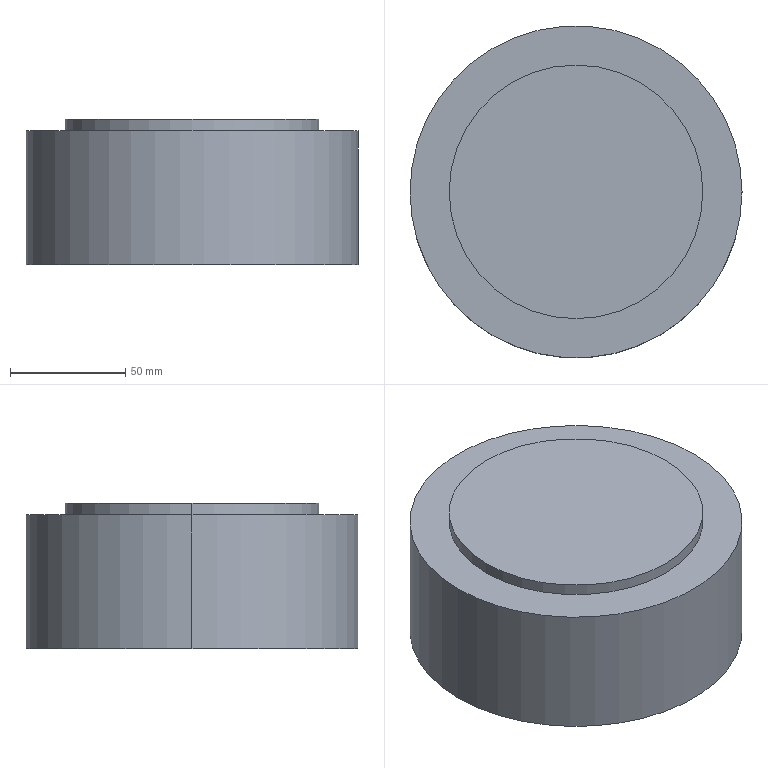Part | SolidWorks | features Extrusion 1, ICE 1 | 1 solid | 7 faces | box 144 x 144 x 63 mm | volume 992106 mm3 | cylinder 4 | plane 3 | commonest cylinder face diameters 110 x2 144 x2
STEP:
#1=CARTESIAN_POINT('',(55.,0.,63.));
#2=VERTEX_POINT('',#1);
#3=CARTESIAN_POINT('',(-55.,0.,63.));
#4=VERTEX_POINT('',#3);
#5=CARTESIAN_POINT('',(0.,0.,63.));
#6=DIRECTION('',(0.,0.,1.));
#7=DIRECTION('',(1.,0.,0.));
#8=AXIS2_PLACEMENT_3D('',#5,#6,#7);
#9=CIRCLE('',#8,55.);
#10=EDGE_CURVE('',#2,#4,#9,.T.);
#11=ORIENTED_EDGE('',*,*,#10,.F.);
#12=CARTESIAN_POINT('',(55.,0.,58.));
#13=VERTEX_POINT('',#12);
#14=CARTESIAN_POINT('',(55.,0.,63.));
#15=DIRECTION('',(0.,0.,-1.));
#16=VECTOR('',#15,1000.);
#17=LINE('',#14,#16);
#18=EDGE_CURVE('',#2,#13,#17,.T.);
#19=ORIENTED_EDGE('',*,*,#18,.T.);
#20=CARTESIAN_POINT('',(-55.,0.,58.));
#21=VERTEX_POINT('',#20);
#22=CARTESIAN_POINT('',(0.,0.,58.));
#23=DIRECTION('',(0.,0.,1.));
#24=DIRECTION('',(1.,0.,0.));
#25=AXIS2_PLACEMENT_3D('',#22,#23,#24);
#26=CIRCLE('',#25,55.);
#27=EDGE_CURVE('',#13,#21,#26,.T.);
#28=ORIENTED_EDGE('',*,*,#27,.T.);
#29=CARTESIAN_POINT('',(-55.,0.,63.));
#30=DIRECTION('',(0.,0.,-1.));
#31=VECTOR('',#30,1000.);
#32=LINE('',#29,#31);
#33=EDGE_CURVE('',#4,#21,#32,.T.);
#34=ORIENTED_EDGE('',*,*,#33,.F.);
#35=EDGE_LOOP('',(#11,#19,#28,#34));
#36=FACE_OUTER_BOUND('',#35,.T.);
#37=CARTESIAN_POINT('',(0.,0.,63.));
#38=DIRECTION('',(0.,0.,-1.));
#39=DIRECTION('',(-1.,0.,0.));
#40=AXIS2_PLACEMENT_3D('',#37,#38,#39);
#41=CYLINDRICAL_SURFACE('',#40,55.);
#42=ADVANCED_FACE('',(#36),#41,.T.);
#43=CARTESIAN_POINT('',(72.,0.,58.));
#44=VERTEX_POINT('',#43);
#45=CARTESIAN_POINT('',(-72.,0.,58.));
#46=VERTEX_POINT('',#45);
#47=CARTESIAN_POINT('',(0.,0.,58.));
#48=DIRECTION('',(0.,0.,1.));
#49=DIRECTION('',(1.,0.,0.));
#50=AXIS2_PLACEMENT_3D('',#47,#48,#49);
#51=CIRCLE('',#50,72.);
#52=EDGE_CURVE('',#44,#46,#51,.T.);
#53=ORIENTED_EDGE('',*,*,#52,.F.);
#54=CARTESIAN_POINT('',(72.,0.,0.));
#55=VERTEX_POINT('',#54);
#56=CARTESIAN_POINT('',(72.,0.,58.));
#57=DIRECTION('',(0.,0.,-1.));
#58=VECTOR('',#57,1000.);
#59=LINE('',#56,#58);
#60=EDGE_CURVE('',#44,#55,#59,.T.);
#61=ORIENTED_EDGE('',*,*,#60,.T.);
#62=CARTESIAN_POINT('',(-72.,0.,0.));
#63=VERTEX_POINT('',#62);
#64=CARTESIAN_POINT('',(0.,0.,0.));
#65=DIRECTION('',(0.,0.,1.));
#66=DIRECTION('',(1.,0.,0.));
#67=AXIS2_PLACEMENT_3D('',#64,#65,#66);
#68=CIRCLE('',#67,72.);
#69=EDGE_CURVE('',#55,#63,#68,.T.);
#70=ORIENTED_EDGE('',*,*,#69,.T.);
#71=CARTESIAN_POINT('',(-72.,0.,58.));
#72=DIRECTION('',(0.,0.,-1.));
#73=VECTOR('',#72,1000.);
#74=LINE('',#71,#73);
#75=EDGE_CURVE('',#46,#63,#74,.T.);
#76=ORIENTED_EDGE('',*,*,#75,.F.);
#77=EDGE_LOOP('',(#53,#61,#70,#76));
#78=FACE_OUTER_BOUND('',#77,.T.);
#79=CARTESIAN_POINT('',(0.,0.,58.));
#80=DIRECTION('',(0.,0.,-1.));
#81=DIRECTION('',(-1.,0.,0.));
#82=AXIS2_PLACEMENT_3D('',#79,#80,#81);
#83=CYLINDRICAL_SURFACE('',#82,72.);
#84=ADVANCED_FACE('',(#78),#83,.T.);
#85=CARTESIAN_POINT('',(0.,0.,58.));
#86=DIRECTION('',(0.,0.,1.));
#87=DIRECTION('',(1.,0.,0.));
#88=AXIS2_PLACEMENT_3D('',#85,#86,#87);
#89=CIRCLE('',#88,72.);
#90=EDGE_CURVE('',#46,#44,#89,.T.);
#91=ORIENTED_EDGE('',*,*,#90,.T.);
#92=ORIENTED_EDGE('',*,*,#52,.T.);
#93=EDGE_LOOP('',(#91,#92));
#94=FACE_OUTER_BOUND('',#93,.T.);
#95=CARTESIAN_POINT('',(0.,0.,58.));
#96=DIRECTION('',(0.,0.,1.));
#97=DIRECTION('',(1.,0.,0.));
#98=AXIS2_PLACEMENT_3D('',#95,#96,#97);
#99=CIRCLE('',#98,55.);
#100=EDGE_CURVE('',#21,#13,#99,.T.);
#101=ORIENTED_EDGE('',*,*,#100,.F.);
#102=ORIENTED_EDGE('',*,*,#27,.F.);
#103=EDGE_LOOP('',(#101,#102));
#104=FACE_BOUND('',#103,.T.);
#105=CARTESIAN_POINT('',(0.,0.,58.));
#106=DIRECTION('',(0.,0.,1.));
#107=DIRECTION('',(1.,0.,0.));
#108=AXIS2_PLACEMENT_3D('',#105,#106,#107);
#109=PLANE('',#108);
#110=ADVANCED_FACE('',(#94,#104),#109,.T.);
#111=ORIENTED_EDGE('',*,*,#60,.F.);
#112=ORIENTED_EDGE('',*,*,#90,.F.);
#113=ORIENTED_EDGE('',*,*,#75,.T.);
#114=CARTESIAN_POINT('',(0.,0.,0.));
#115=DIRECTION('',(0.,0.,1.));
#116=DIRECTION('',(1.,0.,0.));
#117=AXIS2_PLACEMENT_3D('',#114,#115,#116);
#118=CIRCLE('',#117,72.);
#119=EDGE_CURVE('',#63,#55,#118,.T.);
#120=ORIENTED_EDGE('',*,*,#119,.T.);
#121=EDGE_LOOP('',(#111,#112,#113,#120));
#122=FACE_OUTER_BOUND('',#121,.T.);
#123=CARTESIAN_POINT('',(0.,0.,58.));
#124=DIRECTION('',(0.,0.,-1.));
#125=DIRECTION('',(-1.,0.,0.));
#126=AXIS2_PLACEMENT_3D('',#123,#124,#125);
#127=CYLINDRICAL_SURFACE('',#126,72.);
#128=ADVANCED_FACE('',(#122),#127,.T.);
#129=ORIENTED_EDGE('',*,*,#119,.F.);
#130=ORIENTED_EDGE('',*,*,#69,.F.);
#131=EDGE_LOOP('',(#129,#130));
#132=FACE_OUTER_BOUND('',#131,.T.);
#133=CARTESIAN_POINT('',(0.,0.,0.));
#134=DIRECTION('',(0.,0.,1.));
#135=DIRECTION('',(1.,0.,0.));
#136=AXIS2_PLACEMENT_3D('',#133,#134,#135);
#137=PLANE('',#136);
#138=ADVANCED_FACE('',(#132),#137,.F.);
#139=ORIENTED_EDGE('',*,*,#18,.F.);
#140=CARTESIAN_POINT('',(0.,0.,63.));
#141=DIRECTION('',(0.,0.,1.));
#142=DIRECTION('',(1.,0.,0.));
#143=AXIS2_PLACEMENT_3D('',#140,#141,#142);
#144=CIRCLE('',#143,55.);
#145=EDGE_CURVE('',#4,#2,#144,.T.);
#146=ORIENTED_EDGE('',*,*,#145,.F.);
#147=ORIENTED_EDGE('',*,*,#33,.T.);
#148=ORIENTED_EDGE('',*,*,#100,.T.);
#149=EDGE_LOOP('',(#139,#146,#147,#148));
#150=FACE_OUTER_BOUND('',#149,.T.);
#151=CARTESIAN_POINT('',(0.,0.,63.));
#152=DIRECTION('',(0.,0.,-1.));
#153=DIRECTION('',(-1.,0.,0.));
#154=AXIS2_PLACEMENT_3D('',#151,#152,#153);
#155=CYLINDRICAL_SURFACE('',#154,55.);
#156=ADVANCED_FACE('',(#150),#155,.T.);
#157=ORIENTED_EDGE('',*,*,#145,.T.);
#158=ORIENTED_EDGE('',*,*,#10,.T.);
#159=EDGE_LOOP('',(#157,#158));
#160=FACE_OUTER_BOUND('',#159,.T.);
#161=CARTESIAN_POINT('',(0.,0.,63.));
#162=DIRECTION('',(0.,0.,1.));
#163=DIRECTION('',(1.,0.,0.));
#164=AXIS2_PLACEMENT_3D('',#161,#162,#163);
#165=PLANE('',#164);
#166=ADVANCED_FACE('',(#160),#165,.T.);
#167=CLOSED_SHELL('',(#42,#84,#110,#128,#138,#156,#166));
#168=MANIFOLD_SOLID_BREP('',#167);
#169=CARTESIAN_POINT('',(0.,0.,0.));
#170=DIRECTION('',(0.,0.,1.));
#171=DIRECTION('',(1.,0.,0.));
#172=AXIS2_PLACEMENT_3D('',#169,#170,#171);
#173=(LENGTH_UNIT()NAMED_UNIT(*)SI_UNIT(.MILLI.,.METRE.));
#174=UNCERTAINTY_MEASURE_WITH_UNIT(LENGTH_MEASURE(0.00001),#173,'','');
#175=(NAMED_UNIT(*)PLANE_ANGLE_UNIT()SI_UNIT($,.RADIAN.));
#176=(NAMED_UNIT(*)SI_UNIT($,.STERADIAN.)SOLID_ANGLE_UNIT());
#177=(GEOMETRIC_REPRESENTATION_CONTEXT(3)GLOBAL_UNCERTAINTY_ASSIGNED_CONTEXT((#174))GLOBAL_UNIT_ASSIGNED_CONTEXT((#173,#175,#176))REPRESENTATION_CONTEXT('',''));
#178=ADVANCED_BREP_SHAPE_REPRESENTATION('',(#168,#172),#177);